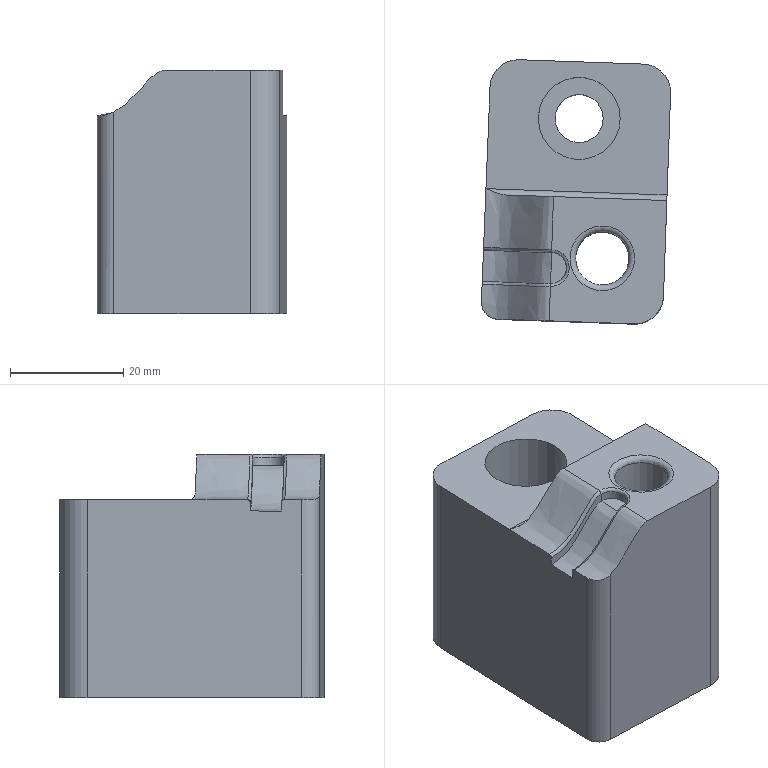Part | NX | features DIE-63 2 | 1 solid | 28 faces | box 33.476 x 46.745 x 43 mm | volume 48597 mm3 | plane 10 | spline 9 | cylinder 8 | torus 1 | commonest cylinder face diameters 10 x3 2 x1 6 x1 8.5 x1 9.44 x1 14.5 x1